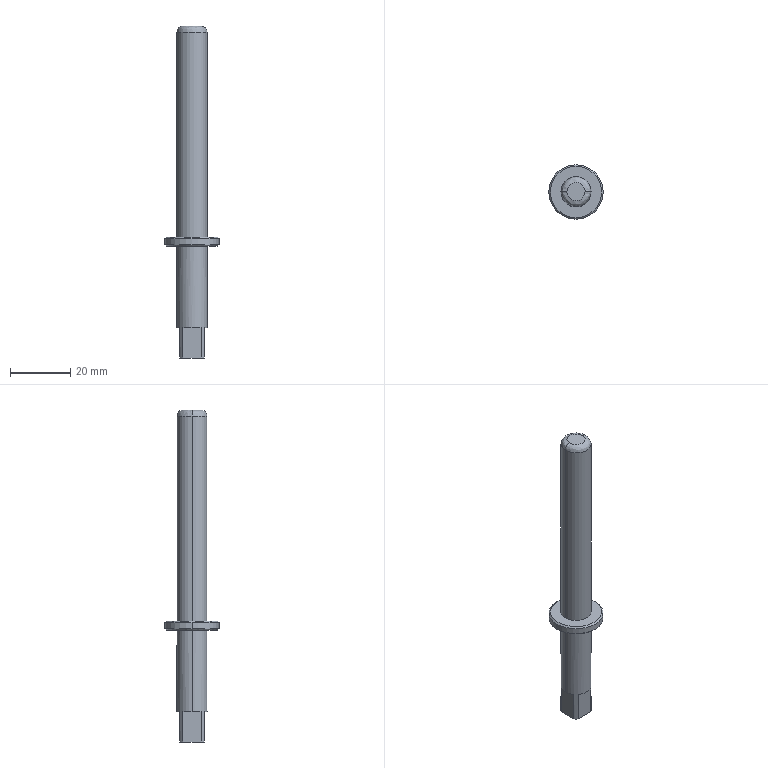Part | STEP file | Adjusting screw | 1 solid | 24 faces | box 18 x 18 x 110 mm | volume 8965 mm3 | plane 12 | cylinder 6 | cone 4 | spline 2 | commonest cylinder face diameters 10 x4 18 x2